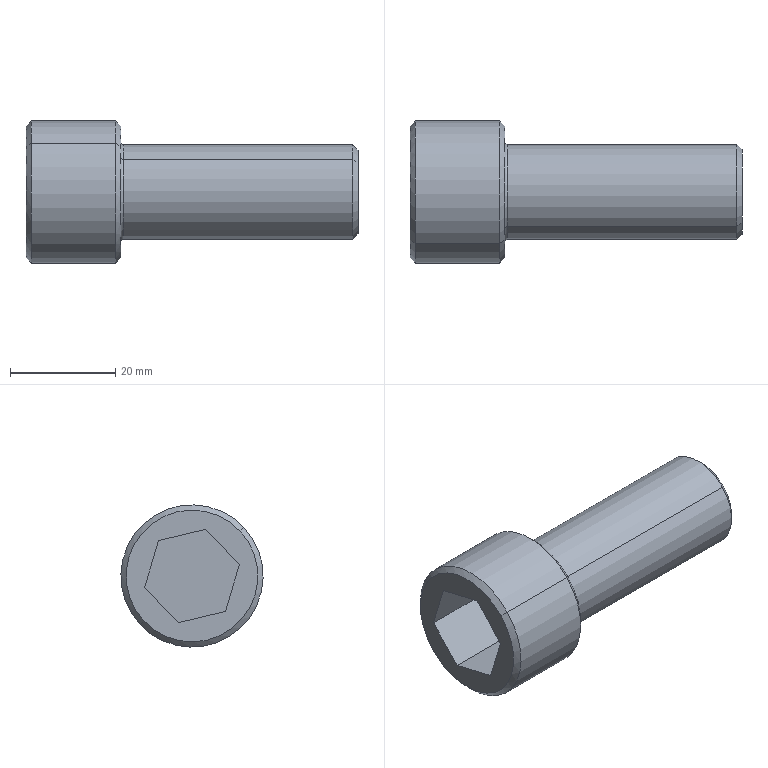Part | NX | features BREP 1 | 1 solid | 22 faces | box 63 x 27 x 27 mm | volume 18990 mm3 | plane 10 | cone 6 | cylinder 4 | torus 2 | commonest cylinder face diameters 18 x2 27 x2
STEP:
#1=CARTESIAN_POINT('',(-624.355,-31.074,25.996));
#2=VERTEX_POINT('',#1);
#3=CARTESIAN_POINT('',(-624.355,-44.894,39.034));
#4=VERTEX_POINT('',#3);
#5=CARTESIAN_POINT('',(-624.355,-37.984,32.515));
#6=DIRECTION('',(-1.,0.,0.));
#7=DIRECTION('',(0.,-0.7274,0.6862));
#8=AXIS2_PLACEMENT_3D('',#5,#6,#7);
#9=CIRCLE('',#8,9.5);
#10=EDGE_CURVE('',#2,#4,#9,.T.);
#11=ORIENTED_EDGE('',*,*,#10,.F.);
#12=CARTESIAN_POINT('',(-623.855,-31.437,26.339));
#13=VERTEX_POINT('',#12);
#14=CARTESIAN_POINT('',(-623.855,-31.074,25.996));
#15=DIRECTION('',(0.,0.6862,0.7274));
#16=DIRECTION('',(0.,0.7274,-0.6862));
#17=AXIS2_PLACEMENT_3D('',#14,#15,#16);
#18=CIRCLE('',#17,0.5);
#19=EDGE_CURVE('',#13,#2,#18,.F.);
#20=ORIENTED_EDGE('',*,*,#19,.F.);
#21=CARTESIAN_POINT('',(-623.855,-44.531,38.691));
#22=VERTEX_POINT('',#21);
#23=CARTESIAN_POINT('',(-623.855,-37.984,32.515));
#24=DIRECTION('',(1.,0.,0.));
#25=DIRECTION('',(0.,-0.7274,0.6862));
#26=AXIS2_PLACEMENT_3D('',#23,#24,#25);
#27=CIRCLE('',#26,9.);
#28=EDGE_CURVE('',#22,#13,#27,.T.);
#29=ORIENTED_EDGE('',*,*,#28,.F.);
#30=CARTESIAN_POINT('',(-623.855,-44.894,39.034));
#31=DIRECTION('',(0.,-0.6862,-0.7274));
#32=DIRECTION('',(1.,0.,0.));
#33=AXIS2_PLACEMENT_3D('',#30,#31,#32);
#34=CIRCLE('',#33,0.5);
#35=EDGE_CURVE('',#22,#4,#34,.F.);
#36=ORIENTED_EDGE('',*,*,#35,.T.);
#37=EDGE_LOOP('',(#11,#20,#29,#36));
#38=FACE_BOUND('',#37,.T.);
#39=CARTESIAN_POINT('',(-623.855,-37.984,32.515));
#40=DIRECTION('',(-1.,0.,0.));
#41=DIRECTION('',(0.,-0.7274,0.6862));
#42=AXIS2_PLACEMENT_3D('',#39,#40,#41);
#43=TOROIDAL_SURFACE('',#42,9.5,0.5);
#44=ADVANCED_FACE('',(#38),#43,.F.);
#45=CARTESIAN_POINT('',(-642.355,-47.077,41.092));
#46=VERTEX_POINT('',#45);
#47=CARTESIAN_POINT('',(-642.355,-28.892,23.937));
#48=VERTEX_POINT('',#47);
#49=CARTESIAN_POINT('',(-642.355,-37.984,32.515));
#50=DIRECTION('',(-1.,0.,0.));
#51=DIRECTION('',(0.,-0.7274,0.6862));
#52=AXIS2_PLACEMENT_3D('',#49,#50,#51);
#53=CIRCLE('',#52,12.5);
#54=EDGE_CURVE('',#46,#48,#53,.T.);
#55=ORIENTED_EDGE('',*,*,#54,.F.);
#56=CARTESIAN_POINT('',(-641.355,-47.804,41.779));
#57=VERTEX_POINT('',#56);
#58=CARTESIAN_POINT('',(-642.355,-47.077,41.092));
#59=DIRECTION('',(0.7071,-0.5144,0.4852));
#60=VECTOR('',#59,1000.);
#61=LINE('',#58,#60);
#62=EDGE_CURVE('',#46,#57,#61,.T.);
#63=ORIENTED_EDGE('',*,*,#62,.T.);
#64=CARTESIAN_POINT('',(-641.355,-28.164,23.251));
#65=VERTEX_POINT('',#64);
#66=CARTESIAN_POINT('',(-641.355,-37.984,32.515));
#67=DIRECTION('',(1.,0.,0.));
#68=DIRECTION('',(0.,-0.7274,0.6862));
#69=AXIS2_PLACEMENT_3D('',#66,#67,#68);
#70=CIRCLE('',#69,13.5);
#71=EDGE_CURVE('',#65,#57,#70,.T.);
#72=ORIENTED_EDGE('',*,*,#71,.F.);
#73=CARTESIAN_POINT('',(-642.355,-28.892,23.937));
#74=DIRECTION('',(0.7071,0.5144,-0.4852));
#75=VECTOR('',#74,1000.);
#76=LINE('',#73,#75);
#77=EDGE_CURVE('',#48,#65,#76,.T.);
#78=ORIENTED_EDGE('',*,*,#77,.F.);
#79=EDGE_LOOP('',(#55,#63,#72,#78));
#80=FACE_BOUND('',#79,.T.);
#81=CARTESIAN_POINT('',(-642.355,-37.984,32.515));
#82=DIRECTION('',(1.,0.,0.));
#83=DIRECTION('',(0.,0.7274,-0.6862));
#84=AXIS2_PLACEMENT_3D('',#81,#82,#83);
#85=CONICAL_SURFACE('',#84,12.5,0.7854);
#86=ADVANCED_FACE('',(#80),#85,.T.);
#87=CARTESIAN_POINT('',(-624.355,-28.892,23.937));
#88=VERTEX_POINT('',#87);
#89=CARTESIAN_POINT('',(-624.355,-47.077,41.092));
#90=VERTEX_POINT('',#89);
#91=CARTESIAN_POINT('',(-624.355,-37.984,32.515));
#92=DIRECTION('',(1.,0.,0.));
#93=DIRECTION('',(0.,-0.7274,0.6862));
#94=AXIS2_PLACEMENT_3D('',#91,#92,#93);
#95=CIRCLE('',#94,12.5);
#96=EDGE_CURVE('',#88,#90,#95,.T.);
#97=ORIENTED_EDGE('',*,*,#96,.F.);
#98=CARTESIAN_POINT('',(-625.355,-28.164,23.251));
#99=VERTEX_POINT('',#98);
#100=CARTESIAN_POINT('',(-625.355,-28.164,23.251));
#101=DIRECTION('',(-0.7071,0.5144,-0.4852));
#102=VECTOR('',#101,1000.);
#103=LINE('',#100,#102);
#104=EDGE_CURVE('',#99,#88,#103,.F.);
#105=ORIENTED_EDGE('',*,*,#104,.F.);
#106=CARTESIAN_POINT('',(-625.355,-47.804,41.779));
#107=VERTEX_POINT('',#106);
#108=CARTESIAN_POINT('',(-625.355,-37.984,32.515));
#109=DIRECTION('',(-1.,0.,0.));
#110=DIRECTION('',(0.,-0.7274,0.6862));
#111=AXIS2_PLACEMENT_3D('',#108,#109,#110);
#112=CIRCLE('',#111,13.5);
#113=EDGE_CURVE('',#107,#99,#112,.T.);
#114=ORIENTED_EDGE('',*,*,#113,.F.);
#115=CARTESIAN_POINT('',(-625.355,-47.804,41.779));
#116=DIRECTION('',(-0.7071,-0.5144,0.4852));
#117=VECTOR('',#116,1000.);
#118=LINE('',#115,#117);
#119=EDGE_CURVE('',#107,#90,#118,.F.);
#120=ORIENTED_EDGE('',*,*,#119,.T.);
#121=EDGE_LOOP('',(#97,#105,#114,#120));
#122=FACE_BOUND('',#121,.T.);
#123=CARTESIAN_POINT('',(-625.355,-37.984,32.515));
#124=DIRECTION('',(-1.,0.,0.));
#125=DIRECTION('',(0.,-0.7274,0.6862));
#126=AXIS2_PLACEMENT_3D('',#123,#124,#125);
#127=CONICAL_SURFACE('',#126,13.5,0.7854);
#128=ADVANCED_FACE('',(#122),#127,.T.);
#129=CARTESIAN_POINT('',(-579.355,-32.165,27.025));
#130=VERTEX_POINT('',#129);
#131=CARTESIAN_POINT('',(-579.355,-43.803,38.004));
#132=VERTEX_POINT('',#131);
#133=CARTESIAN_POINT('',(-579.355,-37.984,32.515));
#134=DIRECTION('',(1.,0.,0.));
#135=DIRECTION('',(0.,-0.7274,0.6862));
#136=AXIS2_PLACEMENT_3D('',#133,#134,#135);
#137=CIRCLE('',#136,8.);
#138=EDGE_CURVE('',#130,#132,#137,.T.);
#139=ORIENTED_EDGE('',*,*,#138,.F.);
#140=CARTESIAN_POINT('',(-580.355,-31.437,26.339));
#141=VERTEX_POINT('',#140);
#142=CARTESIAN_POINT('',(-580.355,-31.437,26.339));
#143=DIRECTION('',(-0.7071,0.5144,-0.4852));
#144=VECTOR('',#143,1000.);
#145=LINE('',#142,#144);
#146=EDGE_CURVE('',#141,#130,#145,.F.);
#147=ORIENTED_EDGE('',*,*,#146,.F.);
#148=CARTESIAN_POINT('',(-580.355,-44.531,38.691));
#149=VERTEX_POINT('',#148);
#150=CARTESIAN_POINT('',(-580.355,-37.984,32.515));
#151=DIRECTION('',(-1.,0.,0.));
#152=DIRECTION('',(0.,-0.7274,0.6862));
#153=AXIS2_PLACEMENT_3D('',#150,#151,#152);
#154=CIRCLE('',#153,9.);
#155=EDGE_CURVE('',#149,#141,#154,.T.);
#156=ORIENTED_EDGE('',*,*,#155,.F.);
#157=CARTESIAN_POINT('',(-580.355,-44.531,38.691));
#158=DIRECTION('',(-0.7071,-0.5144,0.4852));
#159=VECTOR('',#158,1000.);
#160=LINE('',#157,#159);
#161=EDGE_CURVE('',#149,#132,#160,.F.);
#162=ORIENTED_EDGE('',*,*,#161,.T.);
#163=EDGE_LOOP('',(#139,#147,#156,#162));
#164=FACE_BOUND('',#163,.T.);
#165=CARTESIAN_POINT('',(-580.355,-37.984,32.515));
#166=DIRECTION('',(-1.,0.,0.));
#167=DIRECTION('',(0.,-0.7274,0.6862));
#168=AXIS2_PLACEMENT_3D('',#165,#166,#167);
#169=CONICAL_SURFACE('',#168,9.,0.7854);
#170=ADVANCED_FACE('',(#164),#169,.T.);
#171=ORIENTED_EDGE('',*,*,#71,.T.);
#172=CARTESIAN_POINT('',(-642.355,-47.804,41.779));
#173=DIRECTION('',(1.,0.,0.));
#174=VECTOR('',#173,1000.);
#175=LINE('',#172,#174);
#176=EDGE_CURVE('',#57,#107,#175,.T.);
#177=ORIENTED_EDGE('',*,*,#176,.T.);
#178=ORIENTED_EDGE('',*,*,#113,.T.);
#179=CARTESIAN_POINT('',(-642.355,-28.164,23.251));
#180=DIRECTION('',(1.,0.,0.));
#181=VECTOR('',#180,1000.);
#182=LINE('',#179,#181);
#183=EDGE_CURVE('',#65,#99,#182,.T.);
#184=ORIENTED_EDGE('',*,*,#183,.F.);
#185=EDGE_LOOP('',(#171,#177,#178,#184));
#186=FACE_BOUND('',#185,.T.);
#187=CARTESIAN_POINT('',(-642.355,-37.984,32.515));
#188=DIRECTION('',(1.,0.,0.));
#189=DIRECTION('',(0.,0.7274,-0.6862));
#190=AXIS2_PLACEMENT_3D('',#187,#188,#189);
#191=CYLINDRICAL_SURFACE('',#190,13.5);
#192=ADVANCED_FACE('',(#186),#191,.T.);
#193=CARTESIAN_POINT('',(-623.855,-37.984,32.515));
#194=DIRECTION('',(1.,0.,0.));
#195=DIRECTION('',(0.,-0.7274,0.6862));
#196=AXIS2_PLACEMENT_3D('',#193,#194,#195);
#197=CIRCLE('',#196,9.);
#198=EDGE_CURVE('',#13,#22,#197,.T.);
#199=ORIENTED_EDGE('',*,*,#198,.T.);
#200=CARTESIAN_POINT('',(-624.355,-44.531,38.691));
#201=DIRECTION('',(1.,0.,0.));
#202=VECTOR('',#201,1000.);
#203=LINE('',#200,#202);
#204=EDGE_CURVE('',#22,#149,#203,.T.);
#205=ORIENTED_EDGE('',*,*,#204,.T.);
#206=ORIENTED_EDGE('',*,*,#155,.T.);
#207=CARTESIAN_POINT('',(-624.355,-31.437,26.339));
#208=DIRECTION('',(1.,0.,0.));
#209=VECTOR('',#208,1000.);
#210=LINE('',#207,#209);
#211=EDGE_CURVE('',#13,#141,#210,.T.);
#212=ORIENTED_EDGE('',*,*,#211,.F.);
#213=EDGE_LOOP('',(#199,#205,#206,#212));
#214=FACE_BOUND('',#213,.T.);
#215=CARTESIAN_POINT('',(-624.355,-37.984,32.515));
#216=DIRECTION('',(1.,0.,0.));
#217=DIRECTION('',(0.,0.7274,-0.6862));
#218=AXIS2_PLACEMENT_3D('',#215,#216,#217);
#219=CYLINDRICAL_SURFACE('',#218,9.);
#220=ADVANCED_FACE('',(#214),#219,.T.);
#221=ORIENTED_EDGE('',*,*,#204,.F.);
#222=ORIENTED_EDGE('',*,*,#28,.T.);
#223=ORIENTED_EDGE('',*,*,#211,.T.);
#224=CARTESIAN_POINT('',(-580.355,-37.984,32.515));
#225=DIRECTION('',(-1.,0.,0.));
#226=DIRECTION('',(0.,-0.7274,0.6862));
#227=AXIS2_PLACEMENT_3D('',#224,#225,#226);
#228=CIRCLE('',#227,9.);
#229=EDGE_CURVE('',#141,#149,#228,.T.);
#230=ORIENTED_EDGE('',*,*,#229,.T.);
#231=EDGE_LOOP('',(#221,#222,#223,#230));
#232=FACE_BOUND('',#231,.T.);
#233=CARTESIAN_POINT('',(-624.355,-37.984,32.515));
#234=DIRECTION('',(1.,0.,0.));
#235=DIRECTION('',(0.,0.7274,-0.6862));
#236=AXIS2_PLACEMENT_3D('',#233,#234,#235);
#237=CYLINDRICAL_SURFACE('',#236,9.);
#238=ADVANCED_FACE('',(#232),#237,.T.);
#239=CARTESIAN_POINT('',(-579.355,-37.984,32.515));
#240=DIRECTION('',(1.,0.,0.));
#241=DIRECTION('',(0.,-0.7274,0.6862));
#242=AXIS2_PLACEMENT_3D('',#239,#240,#241);
#243=CIRCLE('',#242,8.);
#244=EDGE_CURVE('',#132,#130,#243,.T.);
#245=ORIENTED_EDGE('',*,*,#244,.T.);
#246=ORIENTED_EDGE('',*,*,#138,.T.);
#247=EDGE_LOOP('',(#245,#246));
#248=FACE_BOUND('',#247,.T.);
#249=CARTESIAN_POINT('',(-579.355,-37.984,32.515));
#250=DIRECTION('',(-1.,0.,0.));
#251=DIRECTION('',(0.,-0.7274,0.6862));
#252=AXIS2_PLACEMENT_3D('',#249,#250,#251);
#253=PLANE('',#252);
#254=ADVANCED_FACE('',(#248),#253,.F.);
#255=ORIENTED_EDGE('',*,*,#176,.F.);
#256=CARTESIAN_POINT('',(-641.355,-37.984,32.515));
#257=DIRECTION('',(1.,0.,0.));
#258=DIRECTION('',(0.,-0.7274,0.6862));
#259=AXIS2_PLACEMENT_3D('',#256,#257,#258);
#260=CIRCLE('',#259,13.5);
#261=EDGE_CURVE('',#57,#65,#260,.T.);
#262=ORIENTED_EDGE('',*,*,#261,.T.);
#263=ORIENTED_EDGE('',*,*,#183,.T.);
#264=CARTESIAN_POINT('',(-625.355,-37.984,32.515));
#265=DIRECTION('',(-1.,0.,0.));
#266=DIRECTION('',(0.,-0.7274,0.6862));
#267=AXIS2_PLACEMENT_3D('',#264,#265,#266);
#268=CIRCLE('',#267,13.5);
#269=EDGE_CURVE('',#99,#107,#268,.T.);
#270=ORIENTED_EDGE('',*,*,#269,.T.);
#271=EDGE_LOOP('',(#255,#262,#263,#270));
#272=FACE_BOUND('',#271,.T.);
#273=CARTESIAN_POINT('',(-642.355,-37.984,32.515));
#274=DIRECTION('',(1.,0.,0.));
#275=DIRECTION('',(0.,0.7274,-0.6862));
#276=AXIS2_PLACEMENT_3D('',#273,#274,#275);
#277=CYLINDRICAL_SURFACE('',#276,13.5);
#278=ADVANCED_FACE('',(#272),#277,.T.);
#279=CARTESIAN_POINT('',(-642.355,-37.984,32.515));
#280=DIRECTION('',(-1.,0.,0.));
#281=DIRECTION('',(0.,-0.7274,0.6862));
#282=AXIS2_PLACEMENT_3D('',#279,#280,#281);
#283=CIRCLE('',#282,12.5);
#284=EDGE_CURVE('',#48,#46,#283,.T.);
#285=ORIENTED_EDGE('',*,*,#284,.T.);
#286=ORIENTED_EDGE('',*,*,#54,.T.);
#287=EDGE_LOOP('',(#285,#286));
#288=FACE_BOUND('',#287,.T.);
#289=CARTESIAN_POINT('',(-642.355,-40.634,41.364));
#290=VERTEX_POINT('',#289);
#291=CARTESIAN_POINT('',(-642.355,-31.645,39.234));
#292=VERTEX_POINT('',#291);
#293=CARTESIAN_POINT('',(-642.355,-40.634,41.364));
#294=DIRECTION('',(0.,0.9731,-0.2306));
#295=VECTOR('',#294,1000.);
#296=LINE('',#293,#295);
#297=EDGE_CURVE('',#290,#292,#296,.T.);
#298=ORIENTED_EDGE('',*,*,#297,.F.);
#299=CARTESIAN_POINT('',(-642.355,-46.973,34.645));
#300=VERTEX_POINT('',#299);
#301=CARTESIAN_POINT('',(-642.355,-46.973,34.645));
#302=DIRECTION('',(0.,0.6862,0.7274));
#303=VECTOR('',#302,1000.);
#304=LINE('',#301,#303);
#305=EDGE_CURVE('',#300,#290,#304,.T.);
#306=ORIENTED_EDGE('',*,*,#305,.F.);
#307=CARTESIAN_POINT('',(-642.355,-44.323,25.795));
#308=VERTEX_POINT('',#307);
#309=CARTESIAN_POINT('',(-642.355,-44.323,25.795));
#310=DIRECTION('',(0.,-0.2868,0.958));
#311=VECTOR('',#310,1000.);
#312=LINE('',#309,#311);
#313=EDGE_CURVE('',#308,#300,#312,.T.);
#314=ORIENTED_EDGE('',*,*,#313,.F.);
#315=CARTESIAN_POINT('',(-642.355,-35.334,23.665));
#316=VERTEX_POINT('',#315);
#317=CARTESIAN_POINT('',(-642.355,-35.334,23.665));
#318=DIRECTION('',(0.,-0.9731,0.2306));
#319=VECTOR('',#318,1000.);
#320=LINE('',#317,#319);
#321=EDGE_CURVE('',#316,#308,#320,.T.);
#322=ORIENTED_EDGE('',*,*,#321,.F.);
#323=CARTESIAN_POINT('',(-642.355,-28.995,30.385));
#324=VERTEX_POINT('',#323);
#325=CARTESIAN_POINT('',(-642.355,-28.995,30.385));
#326=DIRECTION('',(0.,-0.6862,-0.7274));
#327=VECTOR('',#326,1000.);
#328=LINE('',#325,#327);
#329=EDGE_CURVE('',#324,#316,#328,.T.);
#330=ORIENTED_EDGE('',*,*,#329,.F.);
#331=CARTESIAN_POINT('',(-642.355,-31.645,39.234));
#332=DIRECTION('',(0.,0.2868,-0.958));
#333=VECTOR('',#332,1000.);
#334=LINE('',#331,#333);
#335=EDGE_CURVE('',#292,#324,#334,.T.);
#336=ORIENTED_EDGE('',*,*,#335,.F.);
#337=EDGE_LOOP('',(#298,#306,#314,#322,#330,#336));
#338=FACE_BOUND('',#337,.T.);
#339=CARTESIAN_POINT('',(-642.355,-37.984,32.515));
#340=DIRECTION('',(-1.,0.,0.));
#341=DIRECTION('',(0.,-0.7274,0.6862));
#342=AXIS2_PLACEMENT_3D('',#339,#340,#341);
#343=PLANE('',#342);
#344=ADVANCED_FACE('',(#288,#338),#343,.T.);
#345=CARTESIAN_POINT('',(-624.355,-37.984,32.515));
#346=DIRECTION('',(-1.,0.,0.));
#347=DIRECTION('',(0.,-0.7274,0.6862));
#348=AXIS2_PLACEMENT_3D('',#345,#346,#347);
#349=CIRCLE('',#348,9.5);
#350=EDGE_CURVE('',#4,#2,#349,.T.);
#351=ORIENTED_EDGE('',*,*,#350,.T.);
#352=ORIENTED_EDGE('',*,*,#10,.T.);
#353=EDGE_LOOP('',(#351,#352));
#354=FACE_BOUND('',#353,.T.);
#355=CARTESIAN_POINT('',(-624.355,-37.984,32.515));
#356=DIRECTION('',(1.,0.,0.));
#357=DIRECTION('',(0.,-0.7274,0.6862));
#358=AXIS2_PLACEMENT_3D('',#355,#356,#357);
#359=CIRCLE('',#358,12.5);
#360=EDGE_CURVE('',#90,#88,#359,.T.);
#361=ORIENTED_EDGE('',*,*,#360,.T.);
#362=ORIENTED_EDGE('',*,*,#96,.T.);
#363=EDGE_LOOP('',(#361,#362));
#364=FACE_BOUND('',#363,.T.);
#365=CARTESIAN_POINT('',(-624.355,-37.984,32.515));
#366=DIRECTION('',(-1.,0.,0.));
#367=DIRECTION('',(0.,-0.7274,0.6862));
#368=AXIS2_PLACEMENT_3D('',#365,#366,#367);
#369=PLANE('',#368);
#370=ADVANCED_FACE('',(#354,#364),#369,.F.);
#371=ORIENTED_EDGE('',*,*,#297,.T.);
#372=CARTESIAN_POINT('',(-630.355,-31.645,39.234));
#373=VERTEX_POINT('',#372);
#374=CARTESIAN_POINT('',(-630.355,-31.645,39.234));
#375=DIRECTION('',(-1.,0.,0.));
#376=VECTOR('',#375,1000.);
#377=LINE('',#374,#376);
#378=EDGE_CURVE('',#373,#292,#377,.T.);
#379=ORIENTED_EDGE('',*,*,#378,.F.);
#380=CARTESIAN_POINT('',(-630.355,-40.634,41.364));
#381=VERTEX_POINT('',#380);
#382=CARTESIAN_POINT('',(-630.355,-40.634,41.364));
#383=DIRECTION('',(0.,0.9731,-0.2306));
#384=VECTOR('',#383,1000.);
#385=LINE('',#382,#384);
#386=EDGE_CURVE('',#381,#373,#385,.T.);
#387=ORIENTED_EDGE('',*,*,#386,.F.);
#388=CARTESIAN_POINT('',(-630.355,-40.634,41.364));
#389=DIRECTION('',(-1.,0.,0.));
#390=VECTOR('',#389,1000.);
#391=LINE('',#388,#390);
#392=EDGE_CURVE('',#381,#290,#391,.T.);
#393=ORIENTED_EDGE('',*,*,#392,.T.);
#394=EDGE_LOOP('',(#371,#379,#387,#393));
#395=FACE_BOUND('',#394,.T.);
#396=CARTESIAN_POINT('',(-630.355,-40.634,41.364));
#397=DIRECTION('',(0.,0.2306,0.9731));
#398=DIRECTION('',(0.,0.9731,-0.2306));
#399=AXIS2_PLACEMENT_3D('',#396,#397,#398);
#400=PLANE('',#399);
#401=ADVANCED_FACE('',(#395),#400,.F.);
#402=ORIENTED_EDGE('',*,*,#305,.T.);
#403=ORIENTED_EDGE('',*,*,#392,.F.);
#404=CARTESIAN_POINT('',(-630.355,-46.973,34.645));
#405=VERTEX_POINT('',#404);
#406=CARTESIAN_POINT('',(-630.355,-46.973,34.645));
#407=DIRECTION('',(0.,0.6862,0.7274));
#408=VECTOR('',#407,1000.);
#409=LINE('',#406,#408);
#410=EDGE_CURVE('',#405,#381,#409,.T.);
#411=ORIENTED_EDGE('',*,*,#410,.F.);
#412=CARTESIAN_POINT('',(-630.355,-46.973,34.645));
#413=DIRECTION('',(-1.,0.,0.));
#414=VECTOR('',#413,1000.);
#415=LINE('',#412,#414);
#416=EDGE_CURVE('',#405,#300,#415,.T.);
#417=ORIENTED_EDGE('',*,*,#416,.T.);
#418=EDGE_LOOP('',(#402,#403,#411,#417));
#419=FACE_BOUND('',#418,.T.);
#420=CARTESIAN_POINT('',(-630.355,-46.973,34.645));
#421=DIRECTION('',(0.,-0.7274,0.6862));
#422=DIRECTION('',(0.,0.6862,0.7274));
#423=AXIS2_PLACEMENT_3D('',#420,#421,#422);
#424=PLANE('',#423);
#425=ADVANCED_FACE('',(#419),#424,.F.);
#426=ORIENTED_EDGE('',*,*,#313,.T.);
#427=ORIENTED_EDGE('',*,*,#416,.F.);
#428=CARTESIAN_POINT('',(-630.355,-44.323,25.795));
#429=VERTEX_POINT('',#428);
#430=CARTESIAN_POINT('',(-630.355,-44.323,25.795));
#431=DIRECTION('',(0.,-0.2868,0.958));
#432=VECTOR('',#431,1000.);
#433=LINE('',#430,#432);
#434=EDGE_CURVE('',#429,#405,#433,.T.);
#435=ORIENTED_EDGE('',*,*,#434,.F.);
#436=CARTESIAN_POINT('',(-630.355,-44.323,25.795));
#437=DIRECTION('',(-1.,0.,0.));
#438=VECTOR('',#437,1000.);
#439=LINE('',#436,#438);
#440=EDGE_CURVE('',#429,#308,#439,.T.);
#441=ORIENTED_EDGE('',*,*,#440,.T.);
#442=EDGE_LOOP('',(#426,#427,#435,#441));
#443=FACE_BOUND('',#442,.T.);
#444=CARTESIAN_POINT('',(-630.355,-44.323,25.795));
#445=DIRECTION('',(0.,-0.958,-0.2868));
#446=DIRECTION('',(0.,-0.2868,0.958));
#447=AXIS2_PLACEMENT_3D('',#444,#445,#446);
#448=PLANE('',#447);
#449=ADVANCED_FACE('',(#443),#448,.F.);
#450=ORIENTED_EDGE('',*,*,#321,.T.);
#451=ORIENTED_EDGE('',*,*,#440,.F.);
#452=CARTESIAN_POINT('',(-630.355,-35.334,23.665));
#453=VERTEX_POINT('',#452);
#454=CARTESIAN_POINT('',(-630.355,-35.334,23.665));
#455=DIRECTION('',(0.,-0.9731,0.2306));
#456=VECTOR('',#455,1000.);
#457=LINE('',#454,#456);
#458=EDGE_CURVE('',#453,#429,#457,.T.);
#459=ORIENTED_EDGE('',*,*,#458,.F.);
#460=CARTESIAN_POINT('',(-630.355,-35.334,23.665));
#461=DIRECTION('',(-1.,0.,0.));
#462=VECTOR('',#461,1000.);
#463=LINE('',#460,#462);
#464=EDGE_CURVE('',#453,#316,#463,.T.);
#465=ORIENTED_EDGE('',*,*,#464,.T.);
#466=EDGE_LOOP('',(#450,#451,#459,#465));
#467=FACE_BOUND('',#466,.T.);
#468=CARTESIAN_POINT('',(-630.355,-35.334,23.665));
#469=DIRECTION('',(0.,-0.2306,-0.9731));
#470=DIRECTION('',(0.,-0.9731,0.2306));
#471=AXIS2_PLACEMENT_3D('',#468,#469,#470);
#472=PLANE('',#471);
#473=ADVANCED_FACE('',(#467),#472,.F.);
#474=ORIENTED_EDGE('',*,*,#329,.T.);
#475=ORIENTED_EDGE('',*,*,#464,.F.);
#476=CARTESIAN_POINT('',(-630.355,-28.995,30.385));
#477=VERTEX_POINT('',#476);
#478=CARTESIAN_POINT('',(-630.355,-28.995,30.385));
#479=DIRECTION('',(0.,-0.6862,-0.7274));
#480=VECTOR('',#479,1000.);
#481=LINE('',#478,#480);
#482=EDGE_CURVE('',#477,#453,#481,.T.);
#483=ORIENTED_EDGE('',*,*,#482,.F.);
#484=CARTESIAN_POINT('',(-630.355,-28.995,30.385));
#485=DIRECTION('',(-1.,0.,0.));
#486=VECTOR('',#485,1000.);
#487=LINE('',#484,#486);
#488=EDGE_CURVE('',#477,#324,#487,.T.);
#489=ORIENTED_EDGE('',*,*,#488,.T.);
#490=EDGE_LOOP('',(#474,#475,#483,#489));
#491=FACE_BOUND('',#490,.T.);
#492=CARTESIAN_POINT('',(-630.355,-28.995,30.385));
#493=DIRECTION('',(0.,0.7274,-0.6862));
#494=DIRECTION('',(0.,-0.6862,-0.7274));
#495=AXIS2_PLACEMENT_3D('',#492,#493,#494);
#496=PLANE('',#495);
#497=ADVANCED_FACE('',(#491),#496,.F.);
#498=ORIENTED_EDGE('',*,*,#335,.T.);
#499=ORIENTED_EDGE('',*,*,#488,.F.);
#500=CARTESIAN_POINT('',(-630.355,-31.645,39.234));
#501=DIRECTION('',(0.,0.2868,-0.958));
#502=VECTOR('',#501,1000.);
#503=LINE('',#500,#502);
#504=EDGE_CURVE('',#373,#477,#503,.T.);
#505=ORIENTED_EDGE('',*,*,#504,.F.);
#506=ORIENTED_EDGE('',*,*,#378,.T.);
#507=EDGE_LOOP('',(#498,#499,#505,#506));
#508=FACE_BOUND('',#507,.T.);
#509=CARTESIAN_POINT('',(-630.355,-31.645,39.234));
#510=DIRECTION('',(0.,0.958,0.2868));
#511=DIRECTION('',(0.,0.2868,-0.958));
#512=AXIS2_PLACEMENT_3D('',#509,#510,#511);
#513=PLANE('',#512);
#514=ADVANCED_FACE('',(#508),#513,.F.);
#515=ORIENTED_EDGE('',*,*,#386,.T.);
#516=ORIENTED_EDGE('',*,*,#504,.T.);
#517=ORIENTED_EDGE('',*,*,#482,.T.);
#518=ORIENTED_EDGE('',*,*,#458,.T.);
#519=ORIENTED_EDGE('',*,*,#434,.T.);
#520=ORIENTED_EDGE('',*,*,#410,.T.);
#521=EDGE_LOOP('',(#515,#516,#517,#518,#519,#520));
#522=FACE_BOUND('',#521,.T.);
#523=CARTESIAN_POINT('',(-630.355,-37.984,32.515));
#524=DIRECTION('',(-1.,0.,0.));
#525=DIRECTION('',(0.,-0.7274,0.6862));
#526=AXIS2_PLACEMENT_3D('',#523,#524,#525);
#527=PLANE('',#526);
#528=ADVANCED_FACE('',(#522),#527,.T.);
#529=ORIENTED_EDGE('',*,*,#146,.T.);
#530=ORIENTED_EDGE('',*,*,#244,.F.);
#531=ORIENTED_EDGE('',*,*,#161,.F.);
#532=ORIENTED_EDGE('',*,*,#229,.F.);
#533=EDGE_LOOP('',(#529,#530,#531,#532));
#534=FACE_BOUND('',#533,.T.);
#535=CARTESIAN_POINT('',(-580.355,-37.984,32.515));
#536=DIRECTION('',(-1.,0.,0.));
#537=DIRECTION('',(0.,-0.7274,0.6862));
#538=AXIS2_PLACEMENT_3D('',#535,#536,#537);
#539=CONICAL_SURFACE('',#538,9.,0.7854);
#540=ADVANCED_FACE('',(#534),#539,.T.);
#541=ORIENTED_EDGE('',*,*,#104,.T.);
#542=ORIENTED_EDGE('',*,*,#360,.F.);
#543=ORIENTED_EDGE('',*,*,#119,.F.);
#544=ORIENTED_EDGE('',*,*,#269,.F.);
#545=EDGE_LOOP('',(#541,#542,#543,#544));
#546=FACE_BOUND('',#545,.T.);
#547=CARTESIAN_POINT('',(-625.355,-37.984,32.515));
#548=DIRECTION('',(-1.,0.,0.));
#549=DIRECTION('',(0.,-0.7274,0.6862));
#550=AXIS2_PLACEMENT_3D('',#547,#548,#549);
#551=CONICAL_SURFACE('',#550,13.5,0.7854);
#552=ADVANCED_FACE('',(#546),#551,.T.);
#553=ORIENTED_EDGE('',*,*,#62,.F.);
#554=ORIENTED_EDGE('',*,*,#284,.F.);
#555=ORIENTED_EDGE('',*,*,#77,.T.);
#556=ORIENTED_EDGE('',*,*,#261,.F.);
#557=EDGE_LOOP('',(#553,#554,#555,#556));
#558=FACE_BOUND('',#557,.T.);
#559=CARTESIAN_POINT('',(-642.355,-37.984,32.515));
#560=DIRECTION('',(1.,0.,0.));
#561=DIRECTION('',(0.,0.7274,-0.6862));
#562=AXIS2_PLACEMENT_3D('',#559,#560,#561);
#563=CONICAL_SURFACE('',#562,12.5,0.7854);
#564=ADVANCED_FACE('',(#558),#563,.T.);
#565=ORIENTED_EDGE('',*,*,#19,.T.);
#566=ORIENTED_EDGE('',*,*,#350,.F.);
#567=ORIENTED_EDGE('',*,*,#35,.F.);
#568=ORIENTED_EDGE('',*,*,#198,.F.);
#569=EDGE_LOOP('',(#565,#566,#567,#568));
#570=FACE_BOUND('',#569,.T.);
#571=CARTESIAN_POINT('',(-623.855,-37.984,32.515));
#572=DIRECTION('',(-1.,0.,0.));
#573=DIRECTION('',(0.,-0.7274,0.6862));
#574=AXIS2_PLACEMENT_3D('',#571,#572,#573);
#575=TOROIDAL_SURFACE('',#574,9.5,0.5);
#576=ADVANCED_FACE('',(#570),#575,.F.);
#577=CLOSED_SHELL('',(#44,#86,#128,#170,#192,#220,#238,#254,#278,#344,#370,#401,#425,#449,#473,#497,#514,#528,#540,#552,#564,#576));
#578=MANIFOLD_SOLID_BREP('',#577);
#579=(LENGTH_UNIT()NAMED_UNIT(*)SI_UNIT(.MILLI.,.METRE.));
#580=UNCERTAINTY_MEASURE_WITH_UNIT(LENGTH_MEASURE(0.00001),#579,'','');
#581=(NAMED_UNIT(*)PLANE_ANGLE_UNIT()SI_UNIT($,.RADIAN.));
#582=(NAMED_UNIT(*)SI_UNIT($,.STERADIAN.)SOLID_ANGLE_UNIT());
#583=(GEOMETRIC_REPRESENTATION_CONTEXT(3)GLOBAL_UNCERTAINTY_ASSIGNED_CONTEXT((#580))GLOBAL_UNIT_ASSIGNED_CONTEXT((#579,#581,#582))REPRESENTATION_CONTEXT('',''));
#584=ADVANCED_BREP_SHAPE_REPRESENTATION('',(#578),#583);